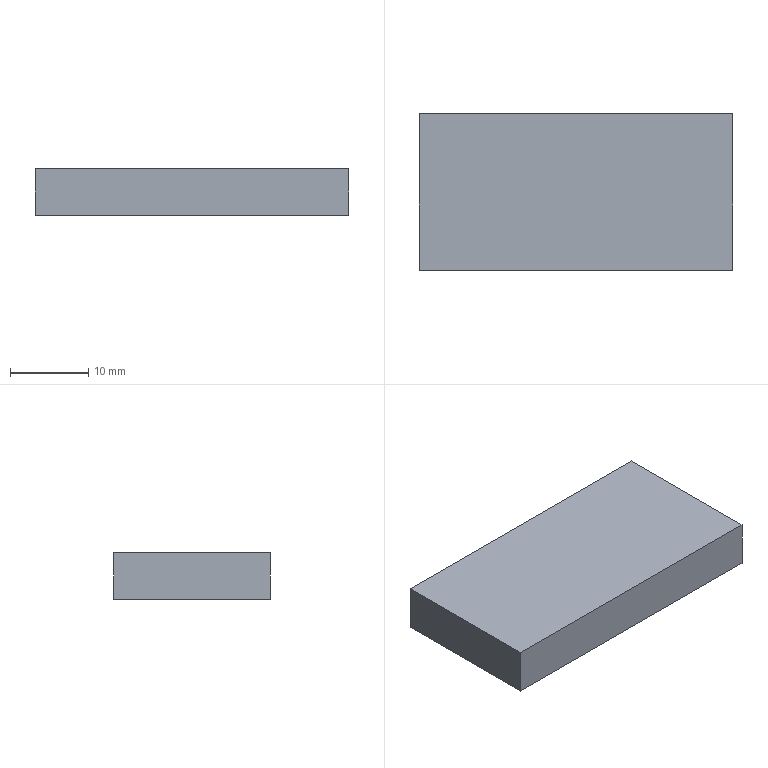Part | STEP file | BCC3 H14_8 | 1 solid | 6 faces | box 40 x 20 x 6 mm | volume 4800 mm3 | plane 6
STEP:
#1=CARTESIAN_POINT('',(0.,0.,0.));
#2=DIRECTION('',(0.,0.,1.));
#3=DIRECTION('',(1.,0.,0.));
#4=AXIS2_PLACEMENT_3D('',#1,#2,#3);
#5=CARTESIAN_POINT('',(-20.,10.,0.));
#6=VERTEX_POINT('',#5);
#7=CARTESIAN_POINT('',(-20.,-10.,0.));
#8=VERTEX_POINT('',#7);
#9=CARTESIAN_POINT('',(-20.,10.,0.));
#10=DIRECTION('',(0.,-1.,0.));
#11=VECTOR('',#10,1.);
#12=LINE('',#9,#11);
#13=CARTESIAN_POINT('',(-20.,10.,-6.));
#14=DIRECTION('',(-1.,0.,0.));
#15=DIRECTION('',(0.,-1.,0.));
#16=AXIS2_PLACEMENT_3D('',#13,#14,#15);
#17=PLANE('',#16);
#18=CARTESIAN_POINT('',(0.,6.));
#19=DIRECTION('',(1.,0.));
#20=VECTOR('',#19,1.);
#21=LINE('',#18,#20);
#22=(GEOMETRIC_REPRESENTATION_CONTEXT(2)PARAMETRIC_REPRESENTATION_CONTEXT()REPRESENTATION_CONTEXT('',''));
#23=DEFINITIONAL_REPRESENTATION('',(#21),#22);
#24=PCURVE('',#17,#23);
#25=CARTESIAN_POINT('',(0.,0.,0.));
#26=DIRECTION('',(0.,0.,1.));
#27=DIRECTION('',(1.,0.,0.));
#28=AXIS2_PLACEMENT_3D('',#25,#26,#27);
#29=PLANE('',#28);
#30=CARTESIAN_POINT('',(-20.,10.));
#31=DIRECTION('',(0.,-1.));
#32=VECTOR('',#31,1.);
#33=LINE('',#30,#32);
#34=(GEOMETRIC_REPRESENTATION_CONTEXT(2)PARAMETRIC_REPRESENTATION_CONTEXT()REPRESENTATION_CONTEXT('',''));
#35=DEFINITIONAL_REPRESENTATION('',(#33),#34);
#36=PCURVE('',#29,#35);
#37=SURFACE_CURVE('',#12,(#24,#36),.PCURVE_S1.);
#38=EDGE_CURVE('',#6,#8,#37,.T.);
#39=ORIENTED_EDGE('',*,*,#38,.F.);
#40=CARTESIAN_POINT('',(-20.,10.,-6.));
#41=VERTEX_POINT('',#40);
#42=CARTESIAN_POINT('',(-20.,10.,-6.));
#43=DIRECTION('',(0.,0.,1.));
#44=VECTOR('',#43,1.);
#45=LINE('',#42,#44);
#46=CARTESIAN_POINT('',(0.,0.));
#47=DIRECTION('',(0.,1.));
#48=VECTOR('',#47,1.);
#49=LINE('',#46,#48);
#50=(GEOMETRIC_REPRESENTATION_CONTEXT(2)PARAMETRIC_REPRESENTATION_CONTEXT()REPRESENTATION_CONTEXT('',''));
#51=DEFINITIONAL_REPRESENTATION('',(#49),#50);
#52=PCURVE('',#17,#51);
#53=CARTESIAN_POINT('',(-20.,10.,-6.));
#54=DIRECTION('',(0.,1.,0.));
#55=DIRECTION('',(0.,0.,1.));
#56=AXIS2_PLACEMENT_3D('',#53,#54,#55);
#57=PLANE('',#56);
#58=CARTESIAN_POINT('',(0.,0.));
#59=DIRECTION('',(1.,0.));
#60=VECTOR('',#59,1.);
#61=LINE('',#58,#60);
#62=(GEOMETRIC_REPRESENTATION_CONTEXT(2)PARAMETRIC_REPRESENTATION_CONTEXT()REPRESENTATION_CONTEXT('',''));
#63=DEFINITIONAL_REPRESENTATION('',(#61),#62);
#64=PCURVE('',#57,#63);
#65=SURFACE_CURVE('',#45,(#52,#64),.PCURVE_S1.);
#66=EDGE_CURVE('',#41,#6,#65,.T.);
#67=ORIENTED_EDGE('',*,*,#66,.F.);
#68=CARTESIAN_POINT('',(-20.,-10.,-6.));
#69=VERTEX_POINT('',#68);
#70=CARTESIAN_POINT('',(-20.,10.,-6.));
#71=DIRECTION('',(0.,-1.,0.));
#72=VECTOR('',#71,1.);
#73=LINE('',#70,#72);
#74=CARTESIAN_POINT('',(0.,0.));
#75=DIRECTION('',(1.,0.));
#76=VECTOR('',#75,1.);
#77=LINE('',#74,#76);
#78=(GEOMETRIC_REPRESENTATION_CONTEXT(2)PARAMETRIC_REPRESENTATION_CONTEXT()REPRESENTATION_CONTEXT('',''));
#79=DEFINITIONAL_REPRESENTATION('',(#77),#78);
#80=PCURVE('',#17,#79);
#81=CARTESIAN_POINT('',(0.,0.,-6.));
#82=DIRECTION('',(0.,0.,1.));
#83=DIRECTION('',(1.,0.,0.));
#84=AXIS2_PLACEMENT_3D('',#81,#82,#83);
#85=PLANE('',#84);
#86=CARTESIAN_POINT('',(-20.,10.));
#87=DIRECTION('',(0.,-1.));
#88=VECTOR('',#87,1.);
#89=LINE('',#86,#88);
#90=(GEOMETRIC_REPRESENTATION_CONTEXT(2)PARAMETRIC_REPRESENTATION_CONTEXT()REPRESENTATION_CONTEXT('',''));
#91=DEFINITIONAL_REPRESENTATION('',(#89),#90);
#92=PCURVE('',#85,#91);
#93=SURFACE_CURVE('',#73,(#80,#92),.PCURVE_S1.);
#94=EDGE_CURVE('',#41,#69,#93,.T.);
#95=ORIENTED_EDGE('',*,*,#94,.T.);
#96=CARTESIAN_POINT('',(-20.,-10.,-6.));
#97=DIRECTION('',(0.,0.,1.));
#98=VECTOR('',#97,1.);
#99=LINE('',#96,#98);
#100=CARTESIAN_POINT('',(20.,0.));
#101=DIRECTION('',(0.,1.));
#102=VECTOR('',#101,1.);
#103=LINE('',#100,#102);
#104=(GEOMETRIC_REPRESENTATION_CONTEXT(2)PARAMETRIC_REPRESENTATION_CONTEXT()REPRESENTATION_CONTEXT('',''));
#105=DEFINITIONAL_REPRESENTATION('',(#103),#104);
#106=PCURVE('',#17,#105);
#107=CARTESIAN_POINT('',(-20.,-10.,-6.));
#108=DIRECTION('',(0.,-1.,0.));
#109=DIRECTION('',(0.,0.,-1.));
#110=AXIS2_PLACEMENT_3D('',#107,#108,#109);
#111=PLANE('',#110);
#112=CARTESIAN_POINT('',(0.,0.));
#113=DIRECTION('',(-1.,0.));
#114=VECTOR('',#113,1.);
#115=LINE('',#112,#114);
#116=(GEOMETRIC_REPRESENTATION_CONTEXT(2)PARAMETRIC_REPRESENTATION_CONTEXT()REPRESENTATION_CONTEXT('',''));
#117=DEFINITIONAL_REPRESENTATION('',(#115),#116);
#118=PCURVE('',#111,#117);
#119=SURFACE_CURVE('',#99,(#106,#118),.PCURVE_S1.);
#120=EDGE_CURVE('',#69,#8,#119,.T.);
#121=ORIENTED_EDGE('',*,*,#120,.T.);
#122=EDGE_LOOP('',(#39,#67,#95,#121));
#123=FACE_BOUND('',#122,.T.);
#124=ADVANCED_FACE('',(#123),#17,.T.);
#125=CARTESIAN_POINT('',(20.,10.,0.));
#126=VERTEX_POINT('',#125);
#127=CARTESIAN_POINT('',(-20.,10.,0.));
#128=DIRECTION('',(-1.,0.,0.));
#129=VECTOR('',#128,1.);
#130=LINE('',#127,#129);
#131=CARTESIAN_POINT('',(6.,0.));
#132=DIRECTION('',(0.,-1.));
#133=VECTOR('',#132,1.);
#134=LINE('',#131,#133);
#135=(GEOMETRIC_REPRESENTATION_CONTEXT(2)PARAMETRIC_REPRESENTATION_CONTEXT()REPRESENTATION_CONTEXT('',''));
#136=DEFINITIONAL_REPRESENTATION('',(#134),#135);
#137=PCURVE('',#57,#136);
#138=CARTESIAN_POINT('',(-20.,10.));
#139=DIRECTION('',(-1.,0.));
#140=VECTOR('',#139,1.);
#141=LINE('',#138,#140);
#142=(GEOMETRIC_REPRESENTATION_CONTEXT(2)PARAMETRIC_REPRESENTATION_CONTEXT()REPRESENTATION_CONTEXT('',''));
#143=DEFINITIONAL_REPRESENTATION('',(#141),#142);
#144=PCURVE('',#29,#143);
#145=SURFACE_CURVE('',#130,(#137,#144),.PCURVE_S1.);
#146=EDGE_CURVE('',#126,#6,#145,.T.);
#147=ORIENTED_EDGE('',*,*,#146,.F.);
#148=CARTESIAN_POINT('',(20.,10.,-6.));
#149=VERTEX_POINT('',#148);
#150=CARTESIAN_POINT('',(20.,10.,-6.));
#151=DIRECTION('',(0.,0.,1.));
#152=VECTOR('',#151,1.);
#153=LINE('',#150,#152);
#154=CARTESIAN_POINT('',(0.,40.));
#155=DIRECTION('',(1.,0.));
#156=VECTOR('',#155,1.);
#157=LINE('',#154,#156);
#158=(GEOMETRIC_REPRESENTATION_CONTEXT(2)PARAMETRIC_REPRESENTATION_CONTEXT()REPRESENTATION_CONTEXT('',''));
#159=DEFINITIONAL_REPRESENTATION('',(#157),#158);
#160=PCURVE('',#57,#159);
#161=CARTESIAN_POINT('',(20.,10.,-6.));
#162=DIRECTION('',(1.,0.,0.));
#163=DIRECTION('',(0.,1.,0.));
#164=AXIS2_PLACEMENT_3D('',#161,#162,#163);
#165=PLANE('',#164);
#166=CARTESIAN_POINT('',(0.,0.));
#167=DIRECTION('',(0.,1.));
#168=VECTOR('',#167,1.);
#169=LINE('',#166,#168);
#170=(GEOMETRIC_REPRESENTATION_CONTEXT(2)PARAMETRIC_REPRESENTATION_CONTEXT()REPRESENTATION_CONTEXT('',''));
#171=DEFINITIONAL_REPRESENTATION('',(#169),#170);
#172=PCURVE('',#165,#171);
#173=SURFACE_CURVE('',#153,(#160,#172),.PCURVE_S1.);
#174=EDGE_CURVE('',#149,#126,#173,.T.);
#175=ORIENTED_EDGE('',*,*,#174,.F.);
#176=CARTESIAN_POINT('',(-20.,10.,-6.));
#177=DIRECTION('',(-1.,0.,0.));
#178=VECTOR('',#177,1.);
#179=LINE('',#176,#178);
#180=CARTESIAN_POINT('',(0.,0.));
#181=DIRECTION('',(0.,-1.));
#182=VECTOR('',#181,1.);
#183=LINE('',#180,#182);
#184=(GEOMETRIC_REPRESENTATION_CONTEXT(2)PARAMETRIC_REPRESENTATION_CONTEXT()REPRESENTATION_CONTEXT('',''));
#185=DEFINITIONAL_REPRESENTATION('',(#183),#184);
#186=PCURVE('',#57,#185);
#187=CARTESIAN_POINT('',(-20.,10.));
#188=DIRECTION('',(-1.,0.));
#189=VECTOR('',#188,1.);
#190=LINE('',#187,#189);
#191=(GEOMETRIC_REPRESENTATION_CONTEXT(2)PARAMETRIC_REPRESENTATION_CONTEXT()REPRESENTATION_CONTEXT('',''));
#192=DEFINITIONAL_REPRESENTATION('',(#190),#191);
#193=PCURVE('',#85,#192);
#194=SURFACE_CURVE('',#179,(#186,#193),.PCURVE_S1.);
#195=EDGE_CURVE('',#149,#41,#194,.T.);
#196=ORIENTED_EDGE('',*,*,#195,.T.);
#197=ORIENTED_EDGE('',*,*,#66,.T.);
#198=EDGE_LOOP('',(#147,#175,#196,#197));
#199=FACE_BOUND('',#198,.T.);
#200=ADVANCED_FACE('',(#199),#57,.T.);
#201=CARTESIAN_POINT('',(20.,-10.,0.));
#202=VERTEX_POINT('',#201);
#203=CARTESIAN_POINT('',(20.,10.,0.));
#204=DIRECTION('',(0.,1.,0.));
#205=VECTOR('',#204,1.);
#206=LINE('',#203,#205);
#207=CARTESIAN_POINT('',(0.,6.));
#208=DIRECTION('',(1.,0.));
#209=VECTOR('',#208,1.);
#210=LINE('',#207,#209);
#211=(GEOMETRIC_REPRESENTATION_CONTEXT(2)PARAMETRIC_REPRESENTATION_CONTEXT()REPRESENTATION_CONTEXT('',''));
#212=DEFINITIONAL_REPRESENTATION('',(#210),#211);
#213=PCURVE('',#165,#212);
#214=CARTESIAN_POINT('',(20.,10.));
#215=DIRECTION('',(0.,1.));
#216=VECTOR('',#215,1.);
#217=LINE('',#214,#216);
#218=(GEOMETRIC_REPRESENTATION_CONTEXT(2)PARAMETRIC_REPRESENTATION_CONTEXT()REPRESENTATION_CONTEXT('',''));
#219=DEFINITIONAL_REPRESENTATION('',(#217),#218);
#220=PCURVE('',#29,#219);
#221=SURFACE_CURVE('',#206,(#213,#220),.PCURVE_S1.);
#222=EDGE_CURVE('',#202,#126,#221,.T.);
#223=ORIENTED_EDGE('',*,*,#222,.F.);
#224=CARTESIAN_POINT('',(20.,-10.,-6.));
#225=VERTEX_POINT('',#224);
#226=CARTESIAN_POINT('',(20.,-10.,-6.));
#227=DIRECTION('',(0.,0.,1.));
#228=VECTOR('',#227,1.);
#229=LINE('',#226,#228);
#230=CARTESIAN_POINT('',(-20.,0.));
#231=DIRECTION('',(0.,1.));
#232=VECTOR('',#231,1.);
#233=LINE('',#230,#232);
#234=(GEOMETRIC_REPRESENTATION_CONTEXT(2)PARAMETRIC_REPRESENTATION_CONTEXT()REPRESENTATION_CONTEXT('',''));
#235=DEFINITIONAL_REPRESENTATION('',(#233),#234);
#236=PCURVE('',#165,#235);
#237=CARTESIAN_POINT('',(0.,40.));
#238=DIRECTION('',(-1.,0.));
#239=VECTOR('',#238,1.);
#240=LINE('',#237,#239);
#241=(GEOMETRIC_REPRESENTATION_CONTEXT(2)PARAMETRIC_REPRESENTATION_CONTEXT()REPRESENTATION_CONTEXT('',''));
#242=DEFINITIONAL_REPRESENTATION('',(#240),#241);
#243=PCURVE('',#111,#242);
#244=SURFACE_CURVE('',#229,(#236,#243),.PCURVE_S1.);
#245=EDGE_CURVE('',#225,#202,#244,.T.);
#246=ORIENTED_EDGE('',*,*,#245,.F.);
#247=CARTESIAN_POINT('',(20.,10.,-6.));
#248=DIRECTION('',(0.,1.,0.));
#249=VECTOR('',#248,1.);
#250=LINE('',#247,#249);
#251=CARTESIAN_POINT('',(0.,0.));
#252=DIRECTION('',(1.,0.));
#253=VECTOR('',#252,1.);
#254=LINE('',#251,#253);
#255=(GEOMETRIC_REPRESENTATION_CONTEXT(2)PARAMETRIC_REPRESENTATION_CONTEXT()REPRESENTATION_CONTEXT('',''));
#256=DEFINITIONAL_REPRESENTATION('',(#254),#255);
#257=PCURVE('',#165,#256);
#258=CARTESIAN_POINT('',(20.,10.));
#259=DIRECTION('',(0.,1.));
#260=VECTOR('',#259,1.);
#261=LINE('',#258,#260);
#262=(GEOMETRIC_REPRESENTATION_CONTEXT(2)PARAMETRIC_REPRESENTATION_CONTEXT()REPRESENTATION_CONTEXT('',''));
#263=DEFINITIONAL_REPRESENTATION('',(#261),#262);
#264=PCURVE('',#85,#263);
#265=SURFACE_CURVE('',#250,(#257,#264),.PCURVE_S1.);
#266=EDGE_CURVE('',#225,#149,#265,.T.);
#267=ORIENTED_EDGE('',*,*,#266,.T.);
#268=ORIENTED_EDGE('',*,*,#174,.T.);
#269=EDGE_LOOP('',(#223,#246,#267,#268));
#270=FACE_BOUND('',#269,.T.);
#271=ADVANCED_FACE('',(#270),#165,.T.);
#272=CARTESIAN_POINT('',(-20.,-10.,0.));
#273=DIRECTION('',(1.,0.,0.));
#274=VECTOR('',#273,1.);
#275=LINE('',#272,#274);
#276=CARTESIAN_POINT('',(-6.,0.));
#277=DIRECTION('',(0.,1.));
#278=VECTOR('',#277,1.);
#279=LINE('',#276,#278);
#280=(GEOMETRIC_REPRESENTATION_CONTEXT(2)PARAMETRIC_REPRESENTATION_CONTEXT()REPRESENTATION_CONTEXT('',''));
#281=DEFINITIONAL_REPRESENTATION('',(#279),#280);
#282=PCURVE('',#111,#281);
#283=CARTESIAN_POINT('',(-20.,-10.));
#284=DIRECTION('',(1.,0.));
#285=VECTOR('',#284,1.);
#286=LINE('',#283,#285);
#287=(GEOMETRIC_REPRESENTATION_CONTEXT(2)PARAMETRIC_REPRESENTATION_CONTEXT()REPRESENTATION_CONTEXT('',''));
#288=DEFINITIONAL_REPRESENTATION('',(#286),#287);
#289=PCURVE('',#29,#288);
#290=SURFACE_CURVE('',#275,(#282,#289),.PCURVE_S1.);
#291=EDGE_CURVE('',#8,#202,#290,.T.);
#292=ORIENTED_EDGE('',*,*,#291,.F.);
#293=ORIENTED_EDGE('',*,*,#120,.F.);
#294=CARTESIAN_POINT('',(-20.,-10.,-6.));
#295=DIRECTION('',(1.,0.,0.));
#296=VECTOR('',#295,1.);
#297=LINE('',#294,#296);
#298=CARTESIAN_POINT('',(0.,0.));
#299=DIRECTION('',(0.,1.));
#300=VECTOR('',#299,1.);
#301=LINE('',#298,#300);
#302=(GEOMETRIC_REPRESENTATION_CONTEXT(2)PARAMETRIC_REPRESENTATION_CONTEXT()REPRESENTATION_CONTEXT('',''));
#303=DEFINITIONAL_REPRESENTATION('',(#301),#302);
#304=PCURVE('',#111,#303);
#305=CARTESIAN_POINT('',(-20.,-10.));
#306=DIRECTION('',(1.,0.));
#307=VECTOR('',#306,1.);
#308=LINE('',#305,#307);
#309=(GEOMETRIC_REPRESENTATION_CONTEXT(2)PARAMETRIC_REPRESENTATION_CONTEXT()REPRESENTATION_CONTEXT('',''));
#310=DEFINITIONAL_REPRESENTATION('',(#308),#309);
#311=PCURVE('',#85,#310);
#312=SURFACE_CURVE('',#297,(#304,#311),.PCURVE_S1.);
#313=EDGE_CURVE('',#69,#225,#312,.T.);
#314=ORIENTED_EDGE('',*,*,#313,.T.);
#315=ORIENTED_EDGE('',*,*,#245,.T.);
#316=EDGE_LOOP('',(#292,#293,#314,#315));
#317=FACE_BOUND('',#316,.T.);
#318=ADVANCED_FACE('',(#317),#111,.T.);
#319=ORIENTED_EDGE('',*,*,#94,.F.);
#320=ORIENTED_EDGE('',*,*,#195,.F.);
#321=ORIENTED_EDGE('',*,*,#266,.F.);
#322=ORIENTED_EDGE('',*,*,#313,.F.);
#323=EDGE_LOOP('',(#319,#320,#321,#322));
#324=FACE_BOUND('',#323,.T.);
#325=ADVANCED_FACE('',(#324),#85,.F.);
#326=ORIENTED_EDGE('',*,*,#38,.T.);
#327=ORIENTED_EDGE('',*,*,#291,.T.);
#328=ORIENTED_EDGE('',*,*,#222,.T.);
#329=ORIENTED_EDGE('',*,*,#146,.T.);
#330=EDGE_LOOP('',(#326,#327,#328,#329));
#331=FACE_BOUND('',#330,.T.);
#332=ADVANCED_FACE('',(#331),#29,.T.);
#333=CLOSED_SHELL('',(#124,#200,#271,#318,#325,#332));
#334=MANIFOLD_SOLID_BREP('',#333);
#335=(LENGTH_UNIT()NAMED_UNIT(*)SI_UNIT(.MILLI.,.METRE.));
#336=UNCERTAINTY_MEASURE_WITH_UNIT(LENGTH_MEASURE(0.0000001),#335,'','');
#337=(NAMED_UNIT(*)PLANE_ANGLE_UNIT()SI_UNIT($,.RADIAN.));
#338=(NAMED_UNIT(*)SI_UNIT($,.STERADIAN.)SOLID_ANGLE_UNIT());
#339=(GEOMETRIC_REPRESENTATION_CONTEXT(3)GLOBAL_UNCERTAINTY_ASSIGNED_CONTEXT((#336))GLOBAL_UNIT_ASSIGNED_CONTEXT((#335,#337,#338))REPRESENTATION_CONTEXT('',''));
#340=ADVANCED_BREP_SHAPE_REPRESENTATION('',(#4,#334),#339);